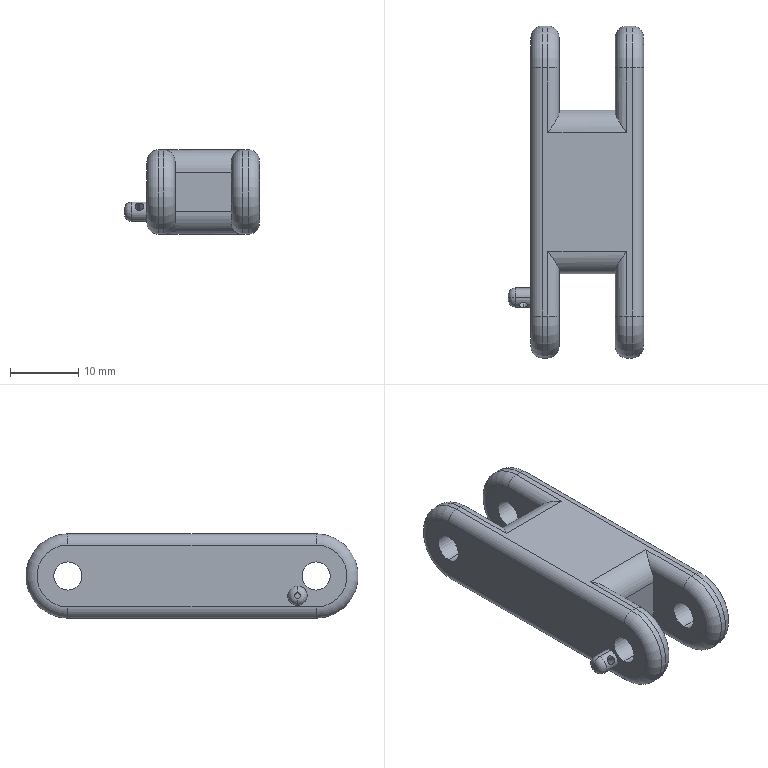Part | SolidWorks | features ICE 4, Fillet 3, 3DProfileFeature 2, Extrusion 1, Scale 1 | 1 solid | 53 faces | box 19.812 x 48.771 x 12.383 mm | volume 6676 mm3 | cylinder 32 | plane 11 | torus 10 | commonest cylinder face diameters 3.302 x12 4.127 x4 4.128 x4 6.604 x4 12.383 x4 1.278 x2